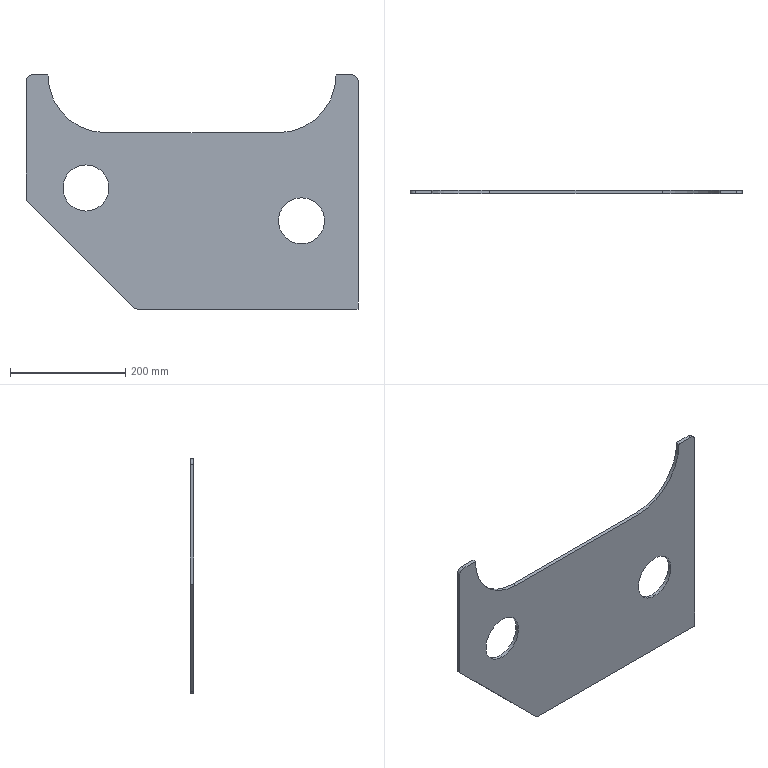Part | SolidWorks | features FlatPattern 1, SMBaseFlange 1, SheetMetal 1 | 1 solid | 18 faces | box 576 x 6 x 406 mm | volume 961136 mm3 | cylinder 9 | plane 9 | commonest cylinder face diameters 80 x4 20 x3 200 x2
STEP:
#1=CARTESIAN_POINT('',(-472.,-6.,170.));
#2=VERTEX_POINT('',#1);
#3=CARTESIAN_POINT('',(-472.,-6.,250.));
#4=VERTEX_POINT('',#3);
#5=CARTESIAN_POINT('',(-472.,-6.,210.));
#6=DIRECTION('',(0.,1.,0.));
#7=DIRECTION('',(0.,0.,1.));
#8=AXIS2_PLACEMENT_3D('',#5,#6,#7);
#9=CIRCLE('',#8,40.);
#10=EDGE_CURVE('',#2,#4,#9,.T.);
#11=ORIENTED_EDGE('',*,*,#10,.F.);
#12=CARTESIAN_POINT('',(-472.,0.,170.));
#13=VERTEX_POINT('',#12);
#14=CARTESIAN_POINT('',(-472.,-6.,170.));
#15=DIRECTION('',(0.,1.,0.));
#16=VECTOR('',#15,1000.);
#17=LINE('',#14,#16);
#18=EDGE_CURVE('',#2,#13,#17,.T.);
#19=ORIENTED_EDGE('',*,*,#18,.T.);
#20=CARTESIAN_POINT('',(-472.,0.,250.));
#21=VERTEX_POINT('',#20);
#22=CARTESIAN_POINT('',(-472.,0.,210.));
#23=DIRECTION('',(0.,1.,0.));
#24=DIRECTION('',(0.,0.,1.));
#25=AXIS2_PLACEMENT_3D('',#22,#23,#24);
#26=CIRCLE('',#25,40.);
#27=EDGE_CURVE('',#13,#21,#26,.T.);
#28=ORIENTED_EDGE('',*,*,#27,.T.);
#29=CARTESIAN_POINT('',(-472.,-6.,250.));
#30=DIRECTION('',(0.,1.,0.));
#31=VECTOR('',#30,1000.);
#32=LINE('',#29,#31);
#33=EDGE_CURVE('',#4,#21,#32,.T.);
#34=ORIENTED_EDGE('',*,*,#33,.F.);
#35=EDGE_LOOP('',(#11,#19,#28,#34));
#36=FACE_OUTER_BOUND('',#35,.T.);
#37=CARTESIAN_POINT('',(-472.,-6.,210.));
#38=DIRECTION('',(0.,1.,0.));
#39=DIRECTION('',(0.,0.,1.));
#40=AXIS2_PLACEMENT_3D('',#37,#38,#39);
#41=CYLINDRICAL_SURFACE('',#40,40.);
#42=ADVANCED_FACE('',(#36),#41,.F.);
#43=CARTESIAN_POINT('',(-98.,-6.,113.));
#44=VERTEX_POINT('',#43);
#45=CARTESIAN_POINT('',(-98.,-6.,193.));
#46=VERTEX_POINT('',#45);
#47=CARTESIAN_POINT('',(-98.,-6.,153.));
#48=DIRECTION('',(0.,1.,0.));
#49=DIRECTION('',(0.,0.,1.));
#50=AXIS2_PLACEMENT_3D('',#47,#48,#49);
#51=CIRCLE('',#50,40.);
#52=EDGE_CURVE('',#44,#46,#51,.T.);
#53=ORIENTED_EDGE('',*,*,#52,.F.);
#54=CARTESIAN_POINT('',(-98.,0.,113.));
#55=VERTEX_POINT('',#54);
#56=CARTESIAN_POINT('',(-98.,-6.,113.));
#57=DIRECTION('',(0.,1.,0.));
#58=VECTOR('',#57,1000.);
#59=LINE('',#56,#58);
#60=EDGE_CURVE('',#44,#55,#59,.T.);
#61=ORIENTED_EDGE('',*,*,#60,.T.);
#62=CARTESIAN_POINT('',(-98.,0.,193.));
#63=VERTEX_POINT('',#62);
#64=CARTESIAN_POINT('',(-98.,0.,153.));
#65=DIRECTION('',(0.,1.,0.));
#66=DIRECTION('',(0.,0.,1.));
#67=AXIS2_PLACEMENT_3D('',#64,#65,#66);
#68=CIRCLE('',#67,40.);
#69=EDGE_CURVE('',#55,#63,#68,.T.);
#70=ORIENTED_EDGE('',*,*,#69,.T.);
#71=CARTESIAN_POINT('',(-98.,-6.,193.));
#72=DIRECTION('',(0.,1.,0.));
#73=VECTOR('',#72,1000.);
#74=LINE('',#71,#73);
#75=EDGE_CURVE('',#46,#63,#74,.T.);
#76=ORIENTED_EDGE('',*,*,#75,.F.);
#77=EDGE_LOOP('',(#53,#61,#70,#76));
#78=FACE_OUTER_BOUND('',#77,.T.);
#79=CARTESIAN_POINT('',(-98.,-6.,153.));
#80=DIRECTION('',(0.,1.,0.));
#81=DIRECTION('',(0.,0.,1.));
#82=AXIS2_PLACEMENT_3D('',#79,#80,#81);
#83=CYLINDRICAL_SURFACE('',#82,40.);
#84=ADVANCED_FACE('',(#78),#83,.F.);
#85=CARTESIAN_POINT('',(0.,0.,396.));
#86=VERTEX_POINT('',#85);
#87=CARTESIAN_POINT('',(0.,0.,0.));
#88=VERTEX_POINT('',#87);
#89=CARTESIAN_POINT('',(0.,0.,396.));
#90=DIRECTION('',(0.,0.,-1.));
#91=VECTOR('',#90,1000.);
#92=LINE('',#89,#91);
#93=EDGE_CURVE('',#86,#88,#92,.T.);
#94=ORIENTED_EDGE('',*,*,#93,.F.);
#95=CARTESIAN_POINT('',(0.,-6.,396.));
#96=VERTEX_POINT('',#95);
#97=CARTESIAN_POINT('',(0.,-6.,396.));
#98=DIRECTION('',(0.,1.,0.));
#99=VECTOR('',#98,1000.);
#100=LINE('',#97,#99);
#101=EDGE_CURVE('',#96,#86,#100,.T.);
#102=ORIENTED_EDGE('',*,*,#101,.F.);
#103=CARTESIAN_POINT('',(0.,-6.,0.));
#104=VERTEX_POINT('',#103);
#105=CARTESIAN_POINT('',(0.,-6.,396.));
#106=DIRECTION('',(0.,0.,-1.));
#107=VECTOR('',#106,1000.);
#108=LINE('',#105,#107);
#109=EDGE_CURVE('',#96,#104,#108,.T.);
#110=ORIENTED_EDGE('',*,*,#109,.T.);
#111=CARTESIAN_POINT('',(0.,-6.,0.));
#112=DIRECTION('',(0.,1.,0.));
#113=VECTOR('',#112,1000.);
#114=LINE('',#111,#113);
#115=EDGE_CURVE('',#104,#88,#114,.T.);
#116=ORIENTED_EDGE('',*,*,#115,.T.);
#117=EDGE_LOOP('',(#94,#102,#110,#116));
#118=FACE_OUTER_BOUND('',#117,.T.);
#119=CARTESIAN_POINT('',(0.,-6.,396.));
#120=DIRECTION('',(1.,0.,0.));
#121=DIRECTION('',(0.,0.,-1.));
#122=AXIS2_PLACEMENT_3D('',#119,#120,#121);
#123=PLANE('',#122);
#124=ADVANCED_FACE('',(#118),#123,.T.);
#125=CARTESIAN_POINT('',(-10.,0.,406.));
#126=VERTEX_POINT('',#125);
#127=CARTESIAN_POINT('',(-10.,0.,396.));
#128=DIRECTION('',(0.,1.,0.));
#129=DIRECTION('',(0.,0.,1.));
#130=AXIS2_PLACEMENT_3D('',#127,#128,#129);
#131=CIRCLE('',#130,10.);
#132=EDGE_CURVE('',#126,#86,#131,.T.);
#133=ORIENTED_EDGE('',*,*,#132,.F.);
#134=CARTESIAN_POINT('',(-10.,-6.,406.));
#135=VERTEX_POINT('',#134);
#136=CARTESIAN_POINT('',(-10.,-6.,406.));
#137=DIRECTION('',(0.,1.,0.));
#138=VECTOR('',#137,1000.);
#139=LINE('',#136,#138);
#140=EDGE_CURVE('',#135,#126,#139,.T.);
#141=ORIENTED_EDGE('',*,*,#140,.F.);
#142=CARTESIAN_POINT('',(-10.,-6.,396.));
#143=DIRECTION('',(0.,1.,0.));
#144=DIRECTION('',(0.,0.,1.));
#145=AXIS2_PLACEMENT_3D('',#142,#143,#144);
#146=CIRCLE('',#145,10.);
#147=EDGE_CURVE('',#135,#96,#146,.T.);
#148=ORIENTED_EDGE('',*,*,#147,.T.);
#149=ORIENTED_EDGE('',*,*,#101,.T.);
#150=EDGE_LOOP('',(#133,#141,#148,#149));
#151=FACE_OUTER_BOUND('',#150,.T.);
#152=CARTESIAN_POINT('',(-10.,-6.,396.));
#153=DIRECTION('',(0.,1.,0.));
#154=DIRECTION('',(0.,0.,1.));
#155=AXIS2_PLACEMENT_3D('',#152,#153,#154);
#156=CYLINDRICAL_SURFACE('',#155,10.);
#157=ADVANCED_FACE('',(#151),#156,.T.);
#158=CARTESIAN_POINT('',(-38.,0.,406.));
#159=VERTEX_POINT('',#158);
#160=CARTESIAN_POINT('',(-38.,0.,406.));
#161=DIRECTION('',(1.,0.,0.));
#162=VECTOR('',#161,1000.);
#163=LINE('',#160,#162);
#164=EDGE_CURVE('',#159,#126,#163,.T.);
#165=ORIENTED_EDGE('',*,*,#164,.F.);
#166=CARTESIAN_POINT('',(-38.,-6.,406.));
#167=VERTEX_POINT('',#166);
#168=CARTESIAN_POINT('',(-38.,-6.,406.));
#169=DIRECTION('',(0.,1.,0.));
#170=VECTOR('',#169,1000.);
#171=LINE('',#168,#170);
#172=EDGE_CURVE('',#167,#159,#171,.T.);
#173=ORIENTED_EDGE('',*,*,#172,.F.);
#174=CARTESIAN_POINT('',(-38.,-6.,406.));
#175=DIRECTION('',(1.,0.,0.));
#176=VECTOR('',#175,1000.);
#177=LINE('',#174,#176);
#178=EDGE_CURVE('',#167,#135,#177,.T.);
#179=ORIENTED_EDGE('',*,*,#178,.T.);
#180=ORIENTED_EDGE('',*,*,#140,.T.);
#181=EDGE_LOOP('',(#165,#173,#179,#180));
#182=FACE_OUTER_BOUND('',#181,.T.);
#183=CARTESIAN_POINT('',(-38.,-6.,406.));
#184=DIRECTION('',(0.,0.,1.));
#185=DIRECTION('',(1.,0.,0.));
#186=AXIS2_PLACEMENT_3D('',#183,#184,#185);
#187=PLANE('',#186);
#188=ADVANCED_FACE('',(#182),#187,.T.);
#189=CARTESIAN_POINT('',(-138.,0.,306.));
#190=VERTEX_POINT('',#189);
#191=CARTESIAN_POINT('',(-138.,0.,406.));
#192=DIRECTION('',(0.,-1.,0.));
#193=DIRECTION('',(0.,0.,1.));
#194=AXIS2_PLACEMENT_3D('',#191,#192,#193);
#195=CIRCLE('',#194,100.);
#196=EDGE_CURVE('',#190,#159,#195,.T.);
#197=ORIENTED_EDGE('',*,*,#196,.F.);
#198=CARTESIAN_POINT('',(-138.,-6.,306.));
#199=VERTEX_POINT('',#198);
#200=CARTESIAN_POINT('',(-138.,-6.,306.));
#201=DIRECTION('',(0.,1.,0.));
#202=VECTOR('',#201,1000.);
#203=LINE('',#200,#202);
#204=EDGE_CURVE('',#199,#190,#203,.T.);
#205=ORIENTED_EDGE('',*,*,#204,.F.);
#206=CARTESIAN_POINT('',(-138.,-6.,406.));
#207=DIRECTION('',(0.,-1.,0.));
#208=DIRECTION('',(0.,0.,1.));
#209=AXIS2_PLACEMENT_3D('',#206,#207,#208);
#210=CIRCLE('',#209,100.);
#211=EDGE_CURVE('',#199,#167,#210,.T.);
#212=ORIENTED_EDGE('',*,*,#211,.T.);
#213=ORIENTED_EDGE('',*,*,#172,.T.);
#214=EDGE_LOOP('',(#197,#205,#212,#213));
#215=FACE_OUTER_BOUND('',#214,.T.);
#216=CARTESIAN_POINT('',(-138.,-6.,406.));
#217=DIRECTION('',(0.,1.,0.));
#218=DIRECTION('',(0.,0.,1.));
#219=AXIS2_PLACEMENT_3D('',#216,#217,#218);
#220=CYLINDRICAL_SURFACE('',#219,100.);
#221=ADVANCED_FACE('',(#215),#220,.F.);
#222=CARTESIAN_POINT('',(-438.,0.,306.));
#223=VERTEX_POINT('',#222);
#224=CARTESIAN_POINT('',(-438.,0.,306.));
#225=DIRECTION('',(1.,0.,0.));
#226=VECTOR('',#225,1000.);
#227=LINE('',#224,#226);
#228=EDGE_CURVE('',#223,#190,#227,.T.);
#229=ORIENTED_EDGE('',*,*,#228,.F.);
#230=CARTESIAN_POINT('',(-438.,-6.,306.));
#231=VERTEX_POINT('',#230);
#232=CARTESIAN_POINT('',(-438.,-6.,306.));
#233=DIRECTION('',(0.,1.,0.));
#234=VECTOR('',#233,1000.);
#235=LINE('',#232,#234);
#236=EDGE_CURVE('',#231,#223,#235,.T.);
#237=ORIENTED_EDGE('',*,*,#236,.F.);
#238=CARTESIAN_POINT('',(-438.,-6.,306.));
#239=DIRECTION('',(1.,0.,0.));
#240=VECTOR('',#239,1000.);
#241=LINE('',#238,#240);
#242=EDGE_CURVE('',#231,#199,#241,.T.);
#243=ORIENTED_EDGE('',*,*,#242,.T.);
#244=ORIENTED_EDGE('',*,*,#204,.T.);
#245=EDGE_LOOP('',(#229,#237,#243,#244));
#246=FACE_OUTER_BOUND('',#245,.T.);
#247=CARTESIAN_POINT('',(-438.,-6.,306.));
#248=DIRECTION('',(0.,0.,1.));
#249=DIRECTION('',(1.,0.,0.));
#250=AXIS2_PLACEMENT_3D('',#247,#248,#249);
#251=PLANE('',#250);
#252=ADVANCED_FACE('',(#246),#251,.T.);
#253=CARTESIAN_POINT('',(-538.,0.,406.));
#254=VERTEX_POINT('',#253);
#255=CARTESIAN_POINT('',(-438.,0.,406.));
#256=DIRECTION('',(0.,-1.,0.));
#257=DIRECTION('',(0.,0.,1.));
#258=AXIS2_PLACEMENT_3D('',#255,#256,#257);
#259=CIRCLE('',#258,100.);
#260=EDGE_CURVE('',#254,#223,#259,.T.);
#261=ORIENTED_EDGE('',*,*,#260,.F.);
#262=CARTESIAN_POINT('',(-538.,-6.,406.));
#263=VERTEX_POINT('',#262);
#264=CARTESIAN_POINT('',(-538.,-6.,406.));
#265=DIRECTION('',(0.,1.,0.));
#266=VECTOR('',#265,1000.);
#267=LINE('',#264,#266);
#268=EDGE_CURVE('',#263,#254,#267,.T.);
#269=ORIENTED_EDGE('',*,*,#268,.F.);
#270=CARTESIAN_POINT('',(-438.,-6.,406.));
#271=DIRECTION('',(0.,-1.,0.));
#272=DIRECTION('',(0.,0.,1.));
#273=AXIS2_PLACEMENT_3D('',#270,#271,#272);
#274=CIRCLE('',#273,100.);
#275=EDGE_CURVE('',#263,#231,#274,.T.);
#276=ORIENTED_EDGE('',*,*,#275,.T.);
#277=ORIENTED_EDGE('',*,*,#236,.T.);
#278=EDGE_LOOP('',(#261,#269,#276,#277));
#279=FACE_OUTER_BOUND('',#278,.T.);
#280=CARTESIAN_POINT('',(-438.,-6.,406.));
#281=DIRECTION('',(0.,1.,0.));
#282=DIRECTION('',(0.,0.,1.));
#283=AXIS2_PLACEMENT_3D('',#280,#281,#282);
#284=CYLINDRICAL_SURFACE('',#283,100.);
#285=ADVANCED_FACE('',(#279),#284,.F.);
#286=CARTESIAN_POINT('',(-566.,0.,406.));
#287=VERTEX_POINT('',#286);
#288=CARTESIAN_POINT('',(-566.,0.,406.));
#289=DIRECTION('',(1.,0.,0.));
#290=VECTOR('',#289,1000.);
#291=LINE('',#288,#290);
#292=EDGE_CURVE('',#287,#254,#291,.T.);
#293=ORIENTED_EDGE('',*,*,#292,.F.);
#294=CARTESIAN_POINT('',(-566.,-6.,406.));
#295=VERTEX_POINT('',#294);
#296=CARTESIAN_POINT('',(-566.,-6.,406.));
#297=DIRECTION('',(0.,1.,0.));
#298=VECTOR('',#297,1000.);
#299=LINE('',#296,#298);
#300=EDGE_CURVE('',#295,#287,#299,.T.);
#301=ORIENTED_EDGE('',*,*,#300,.F.);
#302=CARTESIAN_POINT('',(-566.,-6.,406.));
#303=DIRECTION('',(1.,0.,0.));
#304=VECTOR('',#303,1000.);
#305=LINE('',#302,#304);
#306=EDGE_CURVE('',#295,#263,#305,.T.);
#307=ORIENTED_EDGE('',*,*,#306,.T.);
#308=ORIENTED_EDGE('',*,*,#268,.T.);
#309=EDGE_LOOP('',(#293,#301,#307,#308));
#310=FACE_OUTER_BOUND('',#309,.T.);
#311=CARTESIAN_POINT('',(-566.,-6.,406.));
#312=DIRECTION('',(0.,0.,1.));
#313=DIRECTION('',(1.,0.,0.));
#314=AXIS2_PLACEMENT_3D('',#311,#312,#313);
#315=PLANE('',#314);
#316=ADVANCED_FACE('',(#310),#315,.T.);
#317=CARTESIAN_POINT('',(-576.,0.,396.));
#318=VERTEX_POINT('',#317);
#319=CARTESIAN_POINT('',(-566.,0.,396.));
#320=DIRECTION('',(0.,1.,0.));
#321=DIRECTION('',(0.,0.,1.));
#322=AXIS2_PLACEMENT_3D('',#319,#320,#321);
#323=CIRCLE('',#322,10.);
#324=EDGE_CURVE('',#318,#287,#323,.T.);
#325=ORIENTED_EDGE('',*,*,#324,.F.);
#326=CARTESIAN_POINT('',(-576.,-6.,396.));
#327=VERTEX_POINT('',#326);
#328=CARTESIAN_POINT('',(-576.,-6.,396.));
#329=DIRECTION('',(0.,1.,0.));
#330=VECTOR('',#329,1000.);
#331=LINE('',#328,#330);
#332=EDGE_CURVE('',#327,#318,#331,.T.);
#333=ORIENTED_EDGE('',*,*,#332,.F.);
#334=CARTESIAN_POINT('',(-566.,-6.,396.));
#335=DIRECTION('',(0.,1.,0.));
#336=DIRECTION('',(0.,0.,1.));
#337=AXIS2_PLACEMENT_3D('',#334,#335,#336);
#338=CIRCLE('',#337,10.);
#339=EDGE_CURVE('',#327,#295,#338,.T.);
#340=ORIENTED_EDGE('',*,*,#339,.T.);
#341=ORIENTED_EDGE('',*,*,#300,.T.);
#342=EDGE_LOOP('',(#325,#333,#340,#341));
#343=FACE_OUTER_BOUND('',#342,.T.);
#344=CARTESIAN_POINT('',(-566.,-6.,396.));
#345=DIRECTION('',(0.,1.,0.));
#346=DIRECTION('',(0.,0.,1.));
#347=AXIS2_PLACEMENT_3D('',#344,#345,#346);
#348=CYLINDRICAL_SURFACE('',#347,10.);
#349=ADVANCED_FACE('',(#343),#348,.T.);
#350=CARTESIAN_POINT('',(-576.,0.,189.));
#351=VERTEX_POINT('',#350);
#352=CARTESIAN_POINT('',(-576.,0.,189.));
#353=DIRECTION('',(0.,0.,1.));
#354=VECTOR('',#353,1000.);
#355=LINE('',#352,#354);
#356=EDGE_CURVE('',#351,#318,#355,.T.);
#357=ORIENTED_EDGE('',*,*,#356,.F.);
#358=CARTESIAN_POINT('',(-576.,-6.,189.));
#359=VERTEX_POINT('',#358);
#360=CARTESIAN_POINT('',(-576.,-6.,189.));
#361=DIRECTION('',(0.,1.,0.));
#362=VECTOR('',#361,1000.);
#363=LINE('',#360,#362);
#364=EDGE_CURVE('',#359,#351,#363,.T.);
#365=ORIENTED_EDGE('',*,*,#364,.F.);
#366=CARTESIAN_POINT('',(-576.,-6.,189.));
#367=DIRECTION('',(0.,0.,1.));
#368=VECTOR('',#367,1000.);
#369=LINE('',#366,#368);
#370=EDGE_CURVE('',#359,#327,#369,.T.);
#371=ORIENTED_EDGE('',*,*,#370,.T.);
#372=ORIENTED_EDGE('',*,*,#332,.T.);
#373=EDGE_LOOP('',(#357,#365,#371,#372));
#374=FACE_OUTER_BOUND('',#373,.T.);
#375=CARTESIAN_POINT('',(-576.,-6.,189.));
#376=DIRECTION('',(-1.,0.,0.));
#377=DIRECTION('',(0.,0.,1.));
#378=AXIS2_PLACEMENT_3D('',#375,#376,#377);
#379=PLANE('',#378);
#380=ADVANCED_FACE('',(#374),#379,.T.);
#381=CARTESIAN_POINT('',(-389.929,0.,2.929));
#382=VERTEX_POINT('',#381);
#383=CARTESIAN_POINT('',(-389.929,0.,2.929));
#384=DIRECTION('',(-0.7071,0.,0.7071));
#385=VECTOR('',#384,1000.);
#386=LINE('',#383,#385);
#387=EDGE_CURVE('',#382,#351,#386,.T.);
#388=ORIENTED_EDGE('',*,*,#387,.F.);
#389=CARTESIAN_POINT('',(-389.929,-6.,2.929));
#390=VERTEX_POINT('',#389);
#391=CARTESIAN_POINT('',(-389.929,-6.,2.929));
#392=DIRECTION('',(0.,1.,0.));
#393=VECTOR('',#392,1000.);
#394=LINE('',#391,#393);
#395=EDGE_CURVE('',#390,#382,#394,.T.);
#396=ORIENTED_EDGE('',*,*,#395,.F.);
#397=CARTESIAN_POINT('',(-389.929,-6.,2.929));
#398=DIRECTION('',(-0.7071,0.,0.7071));
#399=VECTOR('',#398,1000.);
#400=LINE('',#397,#399);
#401=EDGE_CURVE('',#390,#359,#400,.T.);
#402=ORIENTED_EDGE('',*,*,#401,.T.);
#403=ORIENTED_EDGE('',*,*,#364,.T.);
#404=EDGE_LOOP('',(#388,#396,#402,#403));
#405=FACE_OUTER_BOUND('',#404,.T.);
#406=CARTESIAN_POINT('',(-389.929,-6.,2.929));
#407=DIRECTION('',(-0.7071,0.,-0.7071));
#408=DIRECTION('',(-0.7071,0.,0.7071));
#409=AXIS2_PLACEMENT_3D('',#406,#407,#408);
#410=PLANE('',#409);
#411=ADVANCED_FACE('',(#405),#410,.T.);
#412=CARTESIAN_POINT('',(-382.858,0.,0.));
#413=VERTEX_POINT('',#412);
#414=CARTESIAN_POINT('',(-382.858,0.,10.));
#415=DIRECTION('',(0.,1.,0.));
#416=DIRECTION('',(0.,0.,1.));
#417=AXIS2_PLACEMENT_3D('',#414,#415,#416);
#418=CIRCLE('',#417,10.);
#419=EDGE_CURVE('',#413,#382,#418,.T.);
#420=ORIENTED_EDGE('',*,*,#419,.F.);
#421=CARTESIAN_POINT('',(-382.858,-6.,0.));
#422=VERTEX_POINT('',#421);
#423=CARTESIAN_POINT('',(-382.858,-6.,0.));
#424=DIRECTION('',(0.,1.,0.));
#425=VECTOR('',#424,1000.);
#426=LINE('',#423,#425);
#427=EDGE_CURVE('',#422,#413,#426,.T.);
#428=ORIENTED_EDGE('',*,*,#427,.F.);
#429=CARTESIAN_POINT('',(-382.858,-6.,10.));
#430=DIRECTION('',(0.,1.,0.));
#431=DIRECTION('',(0.,0.,1.));
#432=AXIS2_PLACEMENT_3D('',#429,#430,#431);
#433=CIRCLE('',#432,10.);
#434=EDGE_CURVE('',#422,#390,#433,.T.);
#435=ORIENTED_EDGE('',*,*,#434,.T.);
#436=ORIENTED_EDGE('',*,*,#395,.T.);
#437=EDGE_LOOP('',(#420,#428,#435,#436));
#438=FACE_OUTER_BOUND('',#437,.T.);
#439=CARTESIAN_POINT('',(-382.858,-6.,10.));
#440=DIRECTION('',(0.,1.,0.));
#441=DIRECTION('',(0.,0.,1.));
#442=AXIS2_PLACEMENT_3D('',#439,#440,#441);
#443=CYLINDRICAL_SURFACE('',#442,10.);
#444=ADVANCED_FACE('',(#438),#443,.T.);
#445=CARTESIAN_POINT('',(0.,0.,0.));
#446=DIRECTION('',(-1.,0.,0.));
#447=VECTOR('',#446,1000.);
#448=LINE('',#445,#447);
#449=EDGE_CURVE('',#88,#413,#448,.T.);
#450=ORIENTED_EDGE('',*,*,#449,.F.);
#451=ORIENTED_EDGE('',*,*,#115,.F.);
#452=CARTESIAN_POINT('',(0.,-6.,0.));
#453=DIRECTION('',(-1.,0.,0.));
#454=VECTOR('',#453,1000.);
#455=LINE('',#452,#454);
#456=EDGE_CURVE('',#104,#422,#455,.T.);
#457=ORIENTED_EDGE('',*,*,#456,.T.);
#458=ORIENTED_EDGE('',*,*,#427,.T.);
#459=EDGE_LOOP('',(#450,#451,#457,#458));
#460=FACE_OUTER_BOUND('',#459,.T.);
#461=CARTESIAN_POINT('',(0.,-6.,0.));
#462=DIRECTION('',(0.,0.,-1.));
#463=DIRECTION('',(-1.,0.,0.));
#464=AXIS2_PLACEMENT_3D('',#461,#462,#463);
#465=PLANE('',#464);
#466=ADVANCED_FACE('',(#460),#465,.T.);
#467=CARTESIAN_POINT('',(-472.,-6.,210.));
#468=DIRECTION('',(0.,1.,0.));
#469=DIRECTION('',(0.,0.,1.));
#470=AXIS2_PLACEMENT_3D('',#467,#468,#469);
#471=CIRCLE('',#470,40.);
#472=EDGE_CURVE('',#4,#2,#471,.T.);
#473=ORIENTED_EDGE('',*,*,#472,.T.);
#474=ORIENTED_EDGE('',*,*,#10,.T.);
#475=EDGE_LOOP('',(#473,#474));
#476=FACE_BOUND('',#475,.T.);
#477=CARTESIAN_POINT('',(-98.,-6.,153.));
#478=DIRECTION('',(0.,1.,0.));
#479=DIRECTION('',(0.,0.,1.));
#480=AXIS2_PLACEMENT_3D('',#477,#478,#479);
#481=CIRCLE('',#480,40.);
#482=EDGE_CURVE('',#46,#44,#481,.T.);
#483=ORIENTED_EDGE('',*,*,#482,.T.);
#484=ORIENTED_EDGE('',*,*,#52,.T.);
#485=EDGE_LOOP('',(#483,#484));
#486=FACE_BOUND('',#485,.T.);
#487=ORIENTED_EDGE('',*,*,#109,.F.);
#488=ORIENTED_EDGE('',*,*,#147,.F.);
#489=ORIENTED_EDGE('',*,*,#178,.F.);
#490=ORIENTED_EDGE('',*,*,#211,.F.);
#491=ORIENTED_EDGE('',*,*,#242,.F.);
#492=ORIENTED_EDGE('',*,*,#275,.F.);
#493=ORIENTED_EDGE('',*,*,#306,.F.);
#494=ORIENTED_EDGE('',*,*,#339,.F.);
#495=ORIENTED_EDGE('',*,*,#370,.F.);
#496=ORIENTED_EDGE('',*,*,#401,.F.);
#497=ORIENTED_EDGE('',*,*,#434,.F.);
#498=ORIENTED_EDGE('',*,*,#456,.F.);
#499=EDGE_LOOP('',(#487,#488,#489,#490,#491,#492,#493,#494,#495,#496,#497,#498));
#500=FACE_OUTER_BOUND('',#499,.T.);
#501=CARTESIAN_POINT('',(-382.858,-6.,10.));
#502=DIRECTION('',(0.,1.,0.));
#503=DIRECTION('',(0.,0.,1.));
#504=AXIS2_PLACEMENT_3D('',#501,#502,#503);
#505=PLANE('',#504);
#506=ADVANCED_FACE('',(#476,#486,#500),#505,.F.);
#507=CARTESIAN_POINT('',(-472.,0.,210.));
#508=DIRECTION('',(0.,1.,0.));
#509=DIRECTION('',(0.,0.,1.));
#510=AXIS2_PLACEMENT_3D('',#507,#508,#509);
#511=CIRCLE('',#510,40.);
#512=EDGE_CURVE('',#21,#13,#511,.T.);
#513=ORIENTED_EDGE('',*,*,#512,.F.);
#514=ORIENTED_EDGE('',*,*,#27,.F.);
#515=EDGE_LOOP('',(#513,#514));
#516=FACE_BOUND('',#515,.T.);
#517=CARTESIAN_POINT('',(-98.,0.,153.));
#518=DIRECTION('',(0.,1.,0.));
#519=DIRECTION('',(0.,0.,1.));
#520=AXIS2_PLACEMENT_3D('',#517,#518,#519);
#521=CIRCLE('',#520,40.);
#522=EDGE_CURVE('',#63,#55,#521,.T.);
#523=ORIENTED_EDGE('',*,*,#522,.F.);
#524=ORIENTED_EDGE('',*,*,#69,.F.);
#525=EDGE_LOOP('',(#523,#524));
#526=FACE_BOUND('',#525,.T.);
#527=ORIENTED_EDGE('',*,*,#93,.T.);
#528=ORIENTED_EDGE('',*,*,#449,.T.);
#529=ORIENTED_EDGE('',*,*,#419,.T.);
#530=ORIENTED_EDGE('',*,*,#387,.T.);
#531=ORIENTED_EDGE('',*,*,#356,.T.);
#532=ORIENTED_EDGE('',*,*,#324,.T.);
#533=ORIENTED_EDGE('',*,*,#292,.T.);
#534=ORIENTED_EDGE('',*,*,#260,.T.);
#535=ORIENTED_EDGE('',*,*,#228,.T.);
#536=ORIENTED_EDGE('',*,*,#196,.T.);
#537=ORIENTED_EDGE('',*,*,#164,.T.);
#538=ORIENTED_EDGE('',*,*,#132,.T.);
#539=EDGE_LOOP('',(#527,#528,#529,#530,#531,#532,#533,#534,#535,#536,#537,#538));
#540=FACE_OUTER_BOUND('',#539,.T.);
#541=CARTESIAN_POINT('',(-382.858,0.,10.));
#542=DIRECTION('',(0.,1.,0.));
#543=DIRECTION('',(0.,0.,1.));
#544=AXIS2_PLACEMENT_3D('',#541,#542,#543);
#545=PLANE('',#544);
#546=ADVANCED_FACE('',(#516,#526,#540),#545,.T.);
#547=ORIENTED_EDGE('',*,*,#60,.F.);
#548=ORIENTED_EDGE('',*,*,#482,.F.);
#549=ORIENTED_EDGE('',*,*,#75,.T.);
#550=ORIENTED_EDGE('',*,*,#522,.T.);
#551=EDGE_LOOP('',(#547,#548,#549,#550));
#552=FACE_OUTER_BOUND('',#551,.T.);
#553=CARTESIAN_POINT('',(-98.,-6.,153.));
#554=DIRECTION('',(0.,1.,0.));
#555=DIRECTION('',(0.,0.,1.));
#556=AXIS2_PLACEMENT_3D('',#553,#554,#555);
#557=CYLINDRICAL_SURFACE('',#556,40.);
#558=ADVANCED_FACE('',(#552),#557,.F.);
#559=ORIENTED_EDGE('',*,*,#18,.F.);
#560=ORIENTED_EDGE('',*,*,#472,.F.);
#561=ORIENTED_EDGE('',*,*,#33,.T.);
#562=ORIENTED_EDGE('',*,*,#512,.T.);
#563=EDGE_LOOP('',(#559,#560,#561,#562));
#564=FACE_OUTER_BOUND('',#563,.T.);
#565=CARTESIAN_POINT('',(-472.,-6.,210.));
#566=DIRECTION('',(0.,1.,0.));
#567=DIRECTION('',(0.,0.,1.));
#568=AXIS2_PLACEMENT_3D('',#565,#566,#567);
#569=CYLINDRICAL_SURFACE('',#568,40.);
#570=ADVANCED_FACE('',(#564),#569,.F.);
#571=CLOSED_SHELL('',(#42,#84,#124,#157,#188,#221,#252,#285,#316,#349,#380,#411,#444,#466,#506,#546,#558,#570));
#572=MANIFOLD_SOLID_BREP('',#571);
#573=CARTESIAN_POINT('',(0.,0.,0.));
#574=DIRECTION('',(0.,0.,1.));
#575=DIRECTION('',(1.,0.,0.));
#576=AXIS2_PLACEMENT_3D('',#573,#574,#575);
#577=(LENGTH_UNIT()NAMED_UNIT(*)SI_UNIT(.MILLI.,.METRE.));
#578=UNCERTAINTY_MEASURE_WITH_UNIT(LENGTH_MEASURE(0.00001),#577,'','');
#579=(NAMED_UNIT(*)PLANE_ANGLE_UNIT()SI_UNIT($,.RADIAN.));
#580=(NAMED_UNIT(*)SI_UNIT($,.STERADIAN.)SOLID_ANGLE_UNIT());
#581=(GEOMETRIC_REPRESENTATION_CONTEXT(3)GLOBAL_UNCERTAINTY_ASSIGNED_CONTEXT((#578))GLOBAL_UNIT_ASSIGNED_CONTEXT((#577,#579,#580))REPRESENTATION_CONTEXT('',''));
#582=ADVANCED_BREP_SHAPE_REPRESENTATION('',(#572,#576),#581);